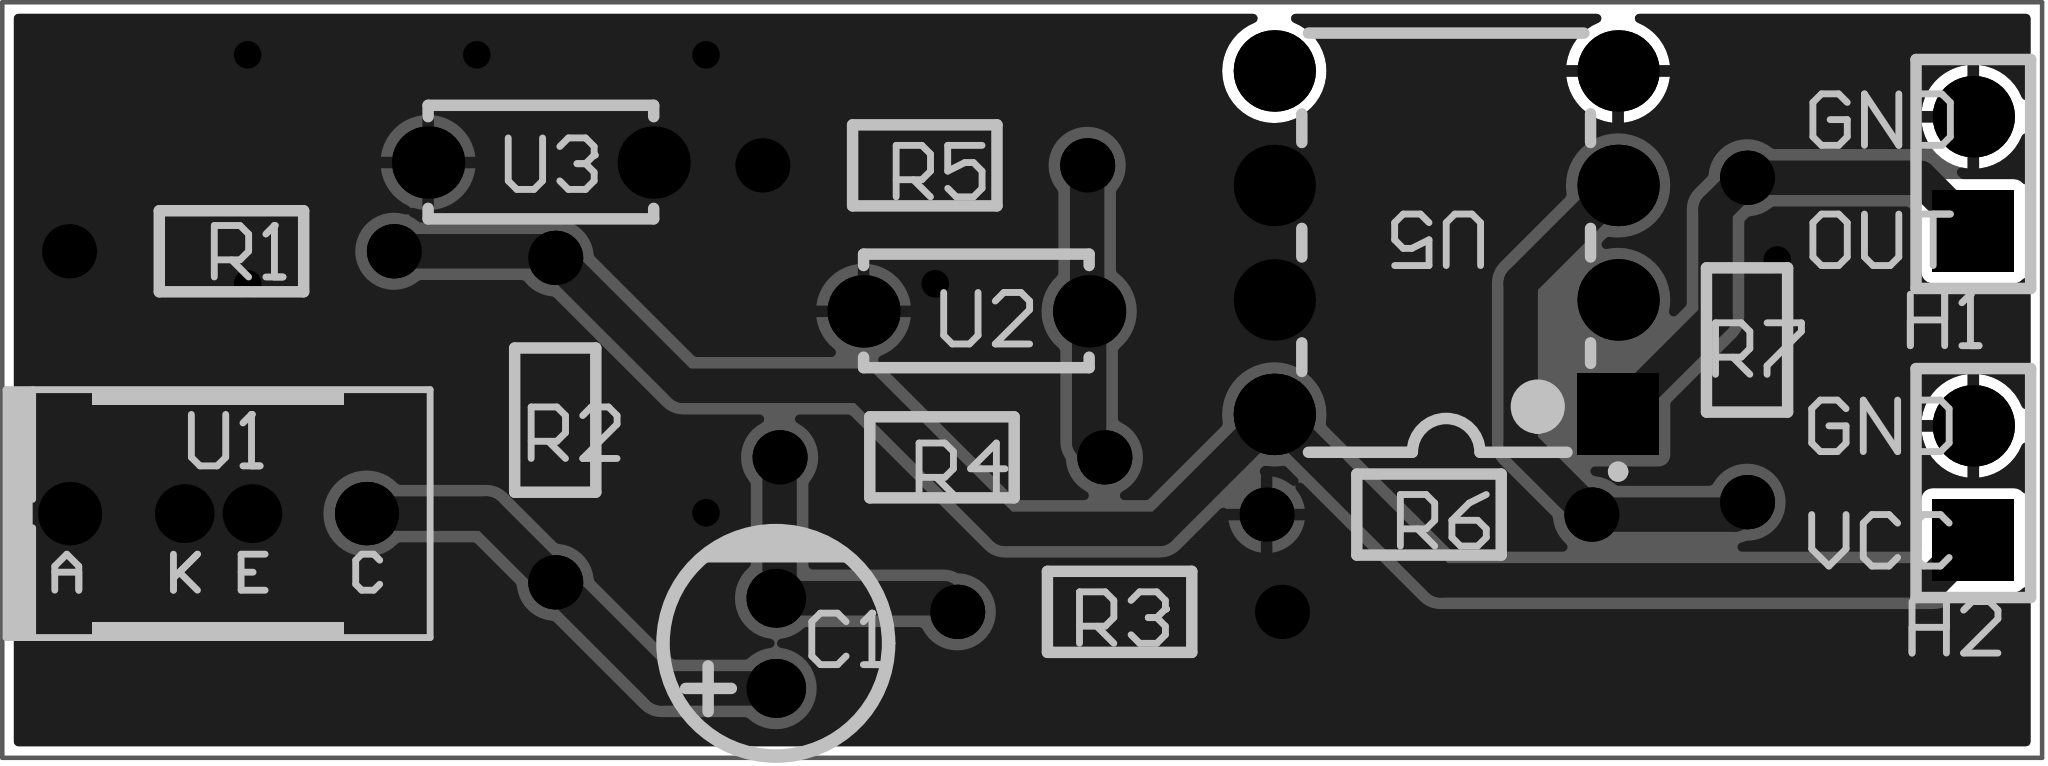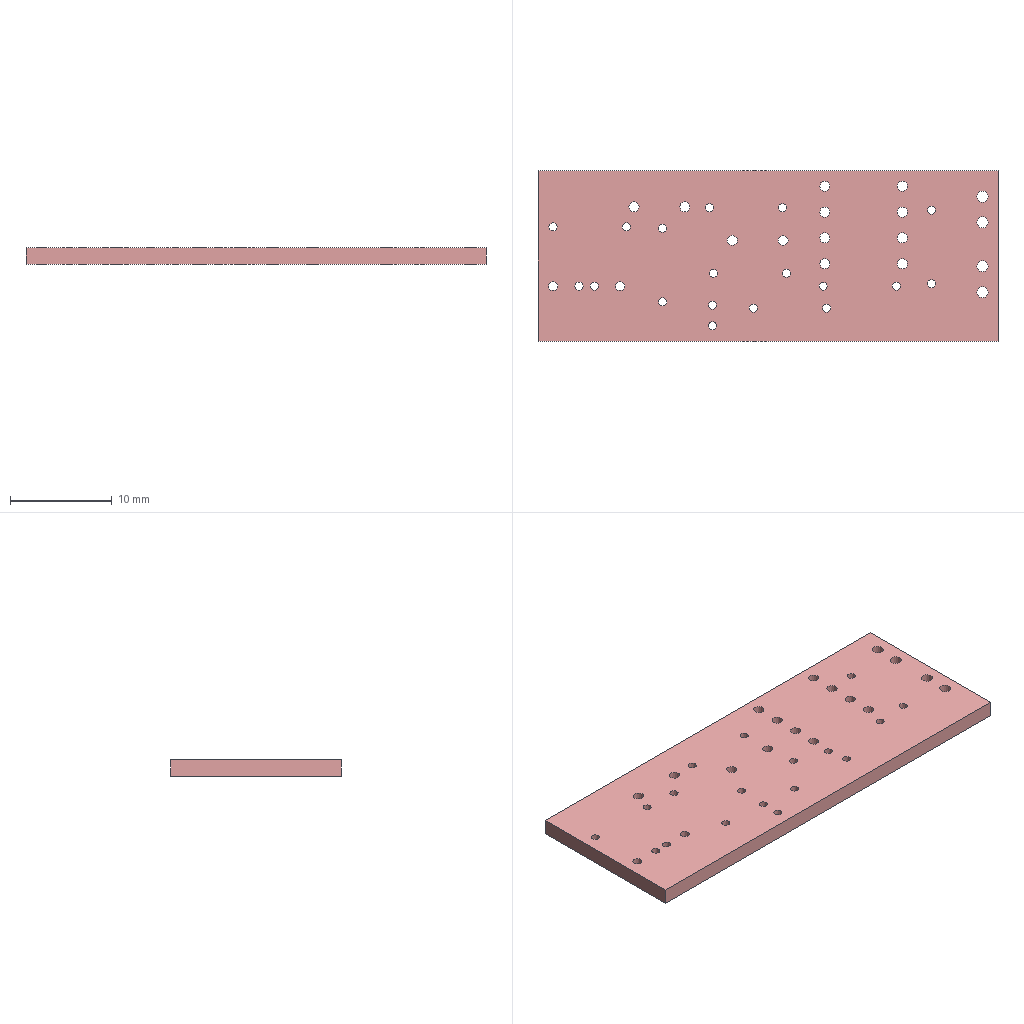Circuit board layout | Altium Designer | box 45.2 x 16.8 x 1.6 mm
Layer stack:
# Altium Designer layer stack of  (unit mm; dielectric type: 0 none, 1 core, 2 prepreg, 3 surface material)
index,name,kind,layer,copper_thickness_mm,dielectric_type,dielectric_thickness_mm,dielectric_material,dielectric_constant
0,Top Paste Mask Layer,other,,,,,,
1,Top Silkscreen Layer,other,,,,,,
2,Top Solder Mask Layer,dielectric,,,3,0.01,,3.3
3,Top Layer,copper,Top Layer,0.035,,,,
4,Dielectric1,dielectric,,,3,1.51,FR4,4.5
5,Bottom Layer,copper,Bottom Layer,0.035,,,,
6,Bottom Solder Mask Layer,dielectric,,,3,0.01,,3.3
7,Bottom Silkscreen Layer,other,,,,,,
8,Bottom Paste Mask Layer,other,,,,,,
# drill layer pairs: low layer,high layer
drill_pair,Top Layer,Bottom Layer
Part placement:
Designator,Comment,Layer,Footprint,Center-X(mm),Center-Y(mm),Rotation
C1,10uF,TopLayer,CAP-TH_BD5.0-P2.00-D0.8-FD-10UF50VC110GL,95.504,81.788,90
H1,,TopLayer,HDR-TH_2P-P2.54-V-M-1,122.047,92.202,90
H2,,TopLayer,HDR-TH_2P-P2.54-V-M-1,122.047,85.344,90
R1,560Ω,TopLayer,Res_1/8W,83.439,90.487,0
R2,560Ω,TopLayer,Res_1/8W,90.615,86.741,90
R3,20KΩ,TopLayer,Res_1/8W,103.124,82.487,180
R4,10kΩ,TopLayer,Res_1/8W,99.187,85.915,0
R5,10kΩ,TopLayer,Res_1/8W,98.806,92.393,180
R6,220Ω,TopLayer,Res_1/8W,109.982,84.645,0
R7,120kΩ,TopLayer,Res_1/8W,117.031,88.519,90
U1,ST188,TopLayer,OPTO-TH_ST188,83.142,84.667,0
U2,105,TopLayer,CAP-TH_L5.0-W2.5-P5.00-D1.0,99.949,89.154,180
U3,105,TopLayer,CAP-TH_L5.0-W2.5-P5.00-D1.0,90.297,92.456,180
U5,LM358N,TopLayer,DIP-8_L9.2-W6.4-P2.54-LS7.6-BL,110.363,90.678,90
Pad and via stacks:
# Altium Designer via and pad stacks of  (unit mm). Each distinct definition once, with the count of objects using it.
# via: kind,start_layer,end_layer,hole_mm,diameter_mm,mode(0 simple;1 top-mid-bottom;2 full stack),diameter_per_layer,count,example_net
# pad: kind,layer,hole_mm,hole_type(0 round;1 square;2 slot),plating,top_size,top_shape(1 round;2 rect;3 octagon;9 rounded rect),mid_size,bottom_size,mode,footprint,size_per_layer,count,example
pad,Multi-Layer,0.8,0,plated,1.3x1.3,1,1.3x1.3,1.3x1.3,0,CAP-TH_BD5.0-P2.00-D0.8-FD-10UF50VC110GL,,2,C1.1
pad,Multi-Layer,1.1,0,plated,1.8x1.8,1,1.8x1.8,1.8x1.8,0,HDR-TH_2P-P2.54-V-M-1,,2,H1.2
pad,Multi-Layer,1.1,0,plated,1.8x1.8,2,1.8x1.8,1.8x1.8,0,HDR-TH_2P-P2.54-V-M-1,,2,H1.1
pad,Multi-Layer,0.8001,0,plated,1.199x1.199,1,1.199x1.199,1.199x1.199,0,Res_1/8W,,14,R1.1
pad,Multi-Layer,0.9,0,plated,1.4x1.4,1,1.4x1.4,1.4x1.4,0,OPTO-TH_ST188,,2,U1.1
pad,Multi-Layer,0.8,0,plated,1.3x1.3,1,1.3x1.3,1.3x1.3,0,OPTO-TH_ST188,,2,U1.2
pad,Multi-Layer,1,0,plated,1.6x1.6,1,1.6x1.6,1.6x1.6,0,CAP-TH_L5.0-W2.5-P5.00-D1.0,,4,U2.1
pad,Multi-Layer,1,0,plated,1.8x1.8,1,1.8x1.8,1.8x1.8,0,DIP-8_L9.2-W6.4-P2.54-LS7.6-BL,,7,U5.8
pad,Multi-Layer,1,0,plated,1.8x1.8,2,1.8x1.8,1.8x1.8,0,DIP-8_L9.2-W6.4-P2.54-LS7.6-BL,,1,U5.1
via,Top Layer,Bottom Layer,0.3048,0.61,0,,7,GND
Copper pours:
name,layer,net,type(0 solid;1 hatched;2 none)
Bottom Layer-GND,Bottom Layer,GND,0
Top Layer-GND,Top Layer,GND,0